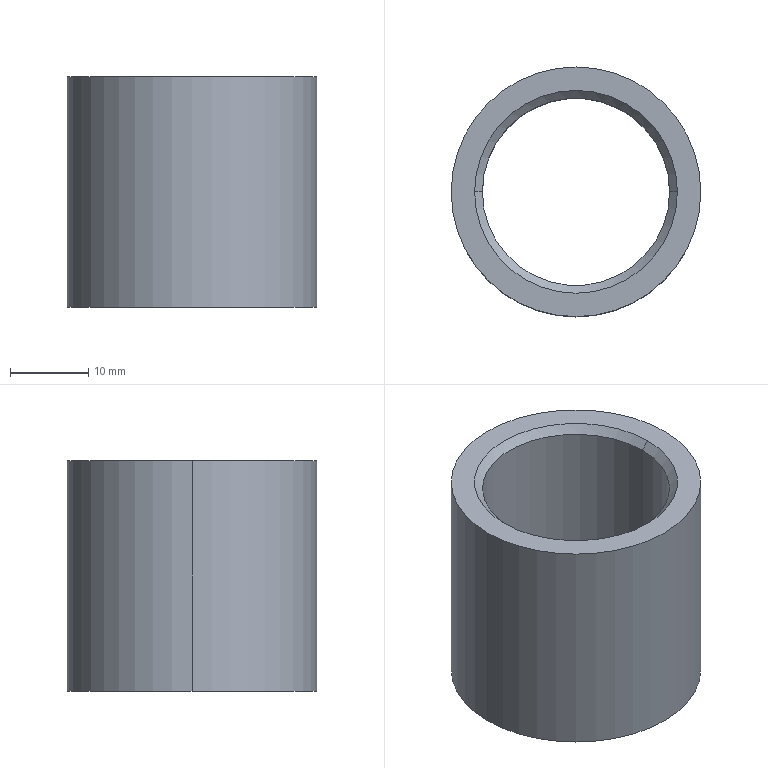Part | STEP file | 塑料轴套内10外20长20 Copy 2 | 1 solid | 10 faces | box 32 x 32 x 29.5 mm | volume 10302 mm3 | cone 4 | cylinder 4 | plane 2 | commonest cylinder face diameters 24 x2 32 x2
STEP:
#1=CARTESIAN_POINT('',(12.,0.,1.));
#2=VERTEX_POINT('',#1);
#3=CARTESIAN_POINT('',(-12.,0.,1.));
#4=VERTEX_POINT('',#3);
#5=CARTESIAN_POINT('',(0.,0.,1.));
#6=DIRECTION('',(0.,0.,-1.));
#7=DIRECTION('',(1.,0.,0.));
#8=AXIS2_PLACEMENT_3D('',#5,#6,#7);
#9=CIRCLE('',#8,12.);
#10=EDGE_CURVE('',#2,#4,#9,.T.);
#11=ORIENTED_EDGE('',*,*,#10,.F.);
#12=CARTESIAN_POINT('',(13.,0.,0.));
#13=VERTEX_POINT('',#12);
#14=CARTESIAN_POINT('',(13.,0.,0.));
#15=DIRECTION('',(0.7071,0.,-0.7071));
#16=VECTOR('',#15,1000.);
#17=LINE('',#14,#16);
#18=EDGE_CURVE('',#2,#13,#17,.T.);
#19=ORIENTED_EDGE('',*,*,#18,.T.);
#20=CARTESIAN_POINT('',(-13.,0.,0.));
#21=VERTEX_POINT('',#20);
#22=CARTESIAN_POINT('',(0.,0.,0.));
#23=DIRECTION('',(0.,0.,1.));
#24=DIRECTION('',(1.,0.,0.));
#25=AXIS2_PLACEMENT_3D('',#22,#23,#24);
#26=CIRCLE('',#25,13.);
#27=EDGE_CURVE('',#21,#13,#26,.T.);
#28=ORIENTED_EDGE('',*,*,#27,.F.);
#29=CARTESIAN_POINT('',(-13.,0.,0.));
#30=DIRECTION('',(-0.7071,0.,-0.7071));
#31=VECTOR('',#30,1000.);
#32=LINE('',#29,#31);
#33=EDGE_CURVE('',#4,#21,#32,.T.);
#34=ORIENTED_EDGE('',*,*,#33,.F.);
#35=EDGE_LOOP('',(#11,#19,#28,#34));
#36=FACE_OUTER_BOUND('',#35,.T.);
#37=CARTESIAN_POINT('',(0.,0.,0.));
#38=DIRECTION('',(0.,0.,-1.));
#39=DIRECTION('',(-1.,0.,0.));
#40=AXIS2_PLACEMENT_3D('',#37,#38,#39);
#41=CONICAL_SURFACE('',#40,13.,0.7854);
#42=ADVANCED_FACE('',(#36),#41,.F.);
#43=CARTESIAN_POINT('',(-12.,0.,28.5));
#44=VERTEX_POINT('',#43);
#45=CARTESIAN_POINT('',(12.,0.,28.5));
#46=VERTEX_POINT('',#45);
#47=CARTESIAN_POINT('',(0.,0.,28.5));
#48=DIRECTION('',(0.,0.,1.));
#49=DIRECTION('',(1.,0.,0.));
#50=AXIS2_PLACEMENT_3D('',#47,#48,#49);
#51=CIRCLE('',#50,12.);
#52=EDGE_CURVE('',#44,#46,#51,.T.);
#53=ORIENTED_EDGE('',*,*,#52,.F.);
#54=CARTESIAN_POINT('',(-13.,0.,29.5));
#55=VERTEX_POINT('',#54);
#56=CARTESIAN_POINT('',(-12.,0.,28.5));
#57=DIRECTION('',(-0.7071,0.,0.7071));
#58=VECTOR('',#57,1000.);
#59=LINE('',#56,#58);
#60=EDGE_CURVE('',#44,#55,#59,.T.);
#61=ORIENTED_EDGE('',*,*,#60,.T.);
#62=CARTESIAN_POINT('',(13.,0.,29.5));
#63=VERTEX_POINT('',#62);
#64=CARTESIAN_POINT('',(0.,0.,29.5));
#65=DIRECTION('',(0.,0.,-1.));
#66=DIRECTION('',(1.,0.,0.));
#67=AXIS2_PLACEMENT_3D('',#64,#65,#66);
#68=CIRCLE('',#67,13.);
#69=EDGE_CURVE('',#63,#55,#68,.T.);
#70=ORIENTED_EDGE('',*,*,#69,.F.);
#71=CARTESIAN_POINT('',(12.,0.,28.5));
#72=DIRECTION('',(0.7071,0.,0.7071));
#73=VECTOR('',#72,1000.);
#74=LINE('',#71,#73);
#75=EDGE_CURVE('',#46,#63,#74,.T.);
#76=ORIENTED_EDGE('',*,*,#75,.F.);
#77=EDGE_LOOP('',(#53,#61,#70,#76));
#78=FACE_OUTER_BOUND('',#77,.T.);
#79=CARTESIAN_POINT('',(0.,0.,28.5));
#80=DIRECTION('',(0.,0.,1.));
#81=DIRECTION('',(1.,0.,0.));
#82=AXIS2_PLACEMENT_3D('',#79,#80,#81);
#83=CONICAL_SURFACE('',#82,12.,0.7854);
#84=ADVANCED_FACE('',(#78),#83,.F.);
#85=ORIENTED_EDGE('',*,*,#52,.T.);
#86=CARTESIAN_POINT('',(12.,0.,29.5));
#87=DIRECTION('',(0.,0.,-1.));
#88=VECTOR('',#87,1000.);
#89=LINE('',#86,#88);
#90=EDGE_CURVE('',#46,#2,#89,.T.);
#91=ORIENTED_EDGE('',*,*,#90,.T.);
#92=ORIENTED_EDGE('',*,*,#10,.T.);
#93=CARTESIAN_POINT('',(-12.,0.,29.5));
#94=DIRECTION('',(0.,0.,-1.));
#95=VECTOR('',#94,1000.);
#96=LINE('',#93,#95);
#97=EDGE_CURVE('',#44,#4,#96,.T.);
#98=ORIENTED_EDGE('',*,*,#97,.F.);
#99=EDGE_LOOP('',(#85,#91,#92,#98));
#100=FACE_OUTER_BOUND('',#99,.T.);
#101=CARTESIAN_POINT('',(0.,0.,29.5));
#102=DIRECTION('',(0.,0.,-1.));
#103=DIRECTION('',(-1.,0.,0.));
#104=AXIS2_PLACEMENT_3D('',#101,#102,#103);
#105=CYLINDRICAL_SURFACE('',#104,12.);
#106=ADVANCED_FACE('',(#100),#105,.F.);
#107=CARTESIAN_POINT('',(16.,0.,29.5));
#108=VERTEX_POINT('',#107);
#109=CARTESIAN_POINT('',(-16.,0.,29.5));
#110=VERTEX_POINT('',#109);
#111=CARTESIAN_POINT('',(0.,0.,29.5));
#112=DIRECTION('',(0.,0.,1.));
#113=DIRECTION('',(1.,0.,0.));
#114=AXIS2_PLACEMENT_3D('',#111,#112,#113);
#115=CIRCLE('',#114,16.);
#116=EDGE_CURVE('',#108,#110,#115,.T.);
#117=ORIENTED_EDGE('',*,*,#116,.F.);
#118=CARTESIAN_POINT('',(16.,0.,0.));
#119=VERTEX_POINT('',#118);
#120=CARTESIAN_POINT('',(16.,0.,29.5));
#121=DIRECTION('',(0.,0.,-1.));
#122=VECTOR('',#121,1000.);
#123=LINE('',#120,#122);
#124=EDGE_CURVE('',#108,#119,#123,.T.);
#125=ORIENTED_EDGE('',*,*,#124,.T.);
#126=CARTESIAN_POINT('',(-16.,0.,0.));
#127=VERTEX_POINT('',#126);
#128=CARTESIAN_POINT('',(0.,0.,0.));
#129=DIRECTION('',(0.,0.,1.));
#130=DIRECTION('',(1.,0.,0.));
#131=AXIS2_PLACEMENT_3D('',#128,#129,#130);
#132=CIRCLE('',#131,16.);
#133=EDGE_CURVE('',#119,#127,#132,.T.);
#134=ORIENTED_EDGE('',*,*,#133,.T.);
#135=CARTESIAN_POINT('',(-16.,0.,29.5));
#136=DIRECTION('',(0.,0.,-1.));
#137=VECTOR('',#136,1000.);
#138=LINE('',#135,#137);
#139=EDGE_CURVE('',#110,#127,#138,.T.);
#140=ORIENTED_EDGE('',*,*,#139,.F.);
#141=EDGE_LOOP('',(#117,#125,#134,#140));
#142=FACE_OUTER_BOUND('',#141,.T.);
#143=CARTESIAN_POINT('',(0.,0.,29.5));
#144=DIRECTION('',(0.,0.,-1.));
#145=DIRECTION('',(-1.,0.,0.));
#146=AXIS2_PLACEMENT_3D('',#143,#144,#145);
#147=CYLINDRICAL_SURFACE('',#146,16.);
#148=ADVANCED_FACE('',(#142),#147,.T.);
#149=ORIENTED_EDGE('',*,*,#69,.T.);
#150=CARTESIAN_POINT('',(0.,0.,29.5));
#151=DIRECTION('',(0.,0.,-1.));
#152=DIRECTION('',(1.,0.,0.));
#153=AXIS2_PLACEMENT_3D('',#150,#151,#152);
#154=CIRCLE('',#153,13.);
#155=EDGE_CURVE('',#55,#63,#154,.T.);
#156=ORIENTED_EDGE('',*,*,#155,.T.);
#157=EDGE_LOOP('',(#149,#156));
#158=FACE_BOUND('',#157,.T.);
#159=CARTESIAN_POINT('',(0.,0.,29.5));
#160=DIRECTION('',(0.,0.,1.));
#161=DIRECTION('',(1.,0.,0.));
#162=AXIS2_PLACEMENT_3D('',#159,#160,#161);
#163=CIRCLE('',#162,16.);
#164=EDGE_CURVE('',#110,#108,#163,.T.);
#165=ORIENTED_EDGE('',*,*,#164,.T.);
#166=ORIENTED_EDGE('',*,*,#116,.T.);
#167=EDGE_LOOP('',(#165,#166));
#168=FACE_OUTER_BOUND('',#167,.T.);
#169=CARTESIAN_POINT('',(0.,0.,29.5));
#170=DIRECTION('',(0.,0.,1.));
#171=DIRECTION('',(1.,0.,0.));
#172=AXIS2_PLACEMENT_3D('',#169,#170,#171);
#173=PLANE('',#172);
#174=ADVANCED_FACE('',(#158,#168),#173,.T.);
#175=ORIENTED_EDGE('',*,*,#27,.T.);
#176=CARTESIAN_POINT('',(0.,0.,0.));
#177=DIRECTION('',(0.,0.,1.));
#178=DIRECTION('',(1.,0.,0.));
#179=AXIS2_PLACEMENT_3D('',#176,#177,#178);
#180=CIRCLE('',#179,13.);
#181=EDGE_CURVE('',#13,#21,#180,.T.);
#182=ORIENTED_EDGE('',*,*,#181,.T.);
#183=EDGE_LOOP('',(#175,#182));
#184=FACE_BOUND('',#183,.T.);
#185=CARTESIAN_POINT('',(0.,0.,0.));
#186=DIRECTION('',(0.,0.,1.));
#187=DIRECTION('',(1.,0.,0.));
#188=AXIS2_PLACEMENT_3D('',#185,#186,#187);
#189=CIRCLE('',#188,16.);
#190=EDGE_CURVE('',#127,#119,#189,.T.);
#191=ORIENTED_EDGE('',*,*,#190,.F.);
#192=ORIENTED_EDGE('',*,*,#133,.F.);
#193=EDGE_LOOP('',(#191,#192));
#194=FACE_OUTER_BOUND('',#193,.T.);
#195=CARTESIAN_POINT('',(0.,0.,0.));
#196=DIRECTION('',(0.,0.,1.));
#197=DIRECTION('',(1.,0.,0.));
#198=AXIS2_PLACEMENT_3D('',#195,#196,#197);
#199=PLANE('',#198);
#200=ADVANCED_FACE('',(#184,#194),#199,.F.);
#201=ORIENTED_EDGE('',*,*,#124,.F.);
#202=ORIENTED_EDGE('',*,*,#164,.F.);
#203=ORIENTED_EDGE('',*,*,#139,.T.);
#204=ORIENTED_EDGE('',*,*,#190,.T.);
#205=EDGE_LOOP('',(#201,#202,#203,#204));
#206=FACE_OUTER_BOUND('',#205,.T.);
#207=CARTESIAN_POINT('',(0.,0.,29.5));
#208=DIRECTION('',(0.,0.,-1.));
#209=DIRECTION('',(-1.,0.,0.));
#210=AXIS2_PLACEMENT_3D('',#207,#208,#209);
#211=CYLINDRICAL_SURFACE('',#210,16.);
#212=ADVANCED_FACE('',(#206),#211,.T.);
#213=ORIENTED_EDGE('',*,*,#90,.F.);
#214=CARTESIAN_POINT('',(0.,0.,28.5));
#215=DIRECTION('',(0.,0.,1.));
#216=DIRECTION('',(1.,0.,0.));
#217=AXIS2_PLACEMENT_3D('',#214,#215,#216);
#218=CIRCLE('',#217,12.);
#219=EDGE_CURVE('',#46,#44,#218,.T.);
#220=ORIENTED_EDGE('',*,*,#219,.T.);
#221=ORIENTED_EDGE('',*,*,#97,.T.);
#222=CARTESIAN_POINT('',(0.,0.,1.));
#223=DIRECTION('',(0.,0.,-1.));
#224=DIRECTION('',(1.,0.,0.));
#225=AXIS2_PLACEMENT_3D('',#222,#223,#224);
#226=CIRCLE('',#225,12.);
#227=EDGE_CURVE('',#4,#2,#226,.T.);
#228=ORIENTED_EDGE('',*,*,#227,.T.);
#229=EDGE_LOOP('',(#213,#220,#221,#228));
#230=FACE_OUTER_BOUND('',#229,.T.);
#231=CARTESIAN_POINT('',(0.,0.,29.5));
#232=DIRECTION('',(0.,0.,-1.));
#233=DIRECTION('',(-1.,0.,0.));
#234=AXIS2_PLACEMENT_3D('',#231,#232,#233);
#235=CYLINDRICAL_SURFACE('',#234,12.);
#236=ADVANCED_FACE('',(#230),#235,.F.);
#237=ORIENTED_EDGE('',*,*,#60,.F.);
#238=ORIENTED_EDGE('',*,*,#219,.F.);
#239=ORIENTED_EDGE('',*,*,#75,.T.);
#240=ORIENTED_EDGE('',*,*,#155,.F.);
#241=EDGE_LOOP('',(#237,#238,#239,#240));
#242=FACE_OUTER_BOUND('',#241,.T.);
#243=CARTESIAN_POINT('',(0.,0.,28.5));
#244=DIRECTION('',(0.,0.,1.));
#245=DIRECTION('',(1.,0.,0.));
#246=AXIS2_PLACEMENT_3D('',#243,#244,#245);
#247=CONICAL_SURFACE('',#246,12.,0.7854);
#248=ADVANCED_FACE('',(#242),#247,.F.);
#249=ORIENTED_EDGE('',*,*,#18,.F.);
#250=ORIENTED_EDGE('',*,*,#227,.F.);
#251=ORIENTED_EDGE('',*,*,#33,.T.);
#252=ORIENTED_EDGE('',*,*,#181,.F.);
#253=EDGE_LOOP('',(#249,#250,#251,#252));
#254=FACE_OUTER_BOUND('',#253,.T.);
#255=CARTESIAN_POINT('',(0.,0.,0.));
#256=DIRECTION('',(0.,0.,-1.));
#257=DIRECTION('',(-1.,0.,0.));
#258=AXIS2_PLACEMENT_3D('',#255,#256,#257);
#259=CONICAL_SURFACE('',#258,13.,0.7854);
#260=ADVANCED_FACE('',(#254),#259,.F.);
#261=CLOSED_SHELL('',(#42,#84,#106,#148,#174,#200,#212,#236,#248,#260));
#262=MANIFOLD_SOLID_BREP('',#261);
#263=CARTESIAN_POINT('',(0.,0.,0.));
#264=DIRECTION('',(0.,0.,1.));
#265=DIRECTION('',(1.,0.,0.));
#266=AXIS2_PLACEMENT_3D('',#263,#264,#265);
#267=(LENGTH_UNIT()NAMED_UNIT(*)SI_UNIT(.MILLI.,.METRE.));
#268=UNCERTAINTY_MEASURE_WITH_UNIT(LENGTH_MEASURE(0.00001),#267,'','');
#269=(NAMED_UNIT(*)PLANE_ANGLE_UNIT()SI_UNIT($,.RADIAN.));
#270=(NAMED_UNIT(*)SI_UNIT($,.STERADIAN.)SOLID_ANGLE_UNIT());
#271=(GEOMETRIC_REPRESENTATION_CONTEXT(3)GLOBAL_UNCERTAINTY_ASSIGNED_CONTEXT((#268))GLOBAL_UNIT_ASSIGNED_CONTEXT((#267,#269,#270))REPRESENTATION_CONTEXT('',''));
#272=ADVANCED_BREP_SHAPE_REPRESENTATION('',(#262,#266),#271);